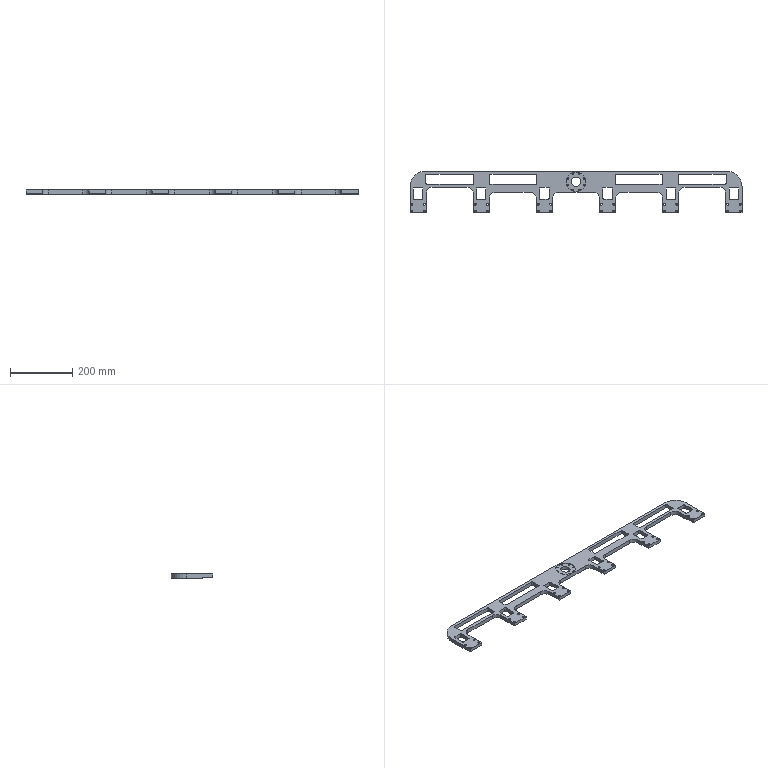Part | 1 solid | 181 faces | box 1068 x 134 x 13 mm | volume 740081 mm3 | cylinder 94 | plane 87 | commonest cylinder face diameters 6 x40 6.5 x24 40 x10 4.5 x8 8 x8 100 x2